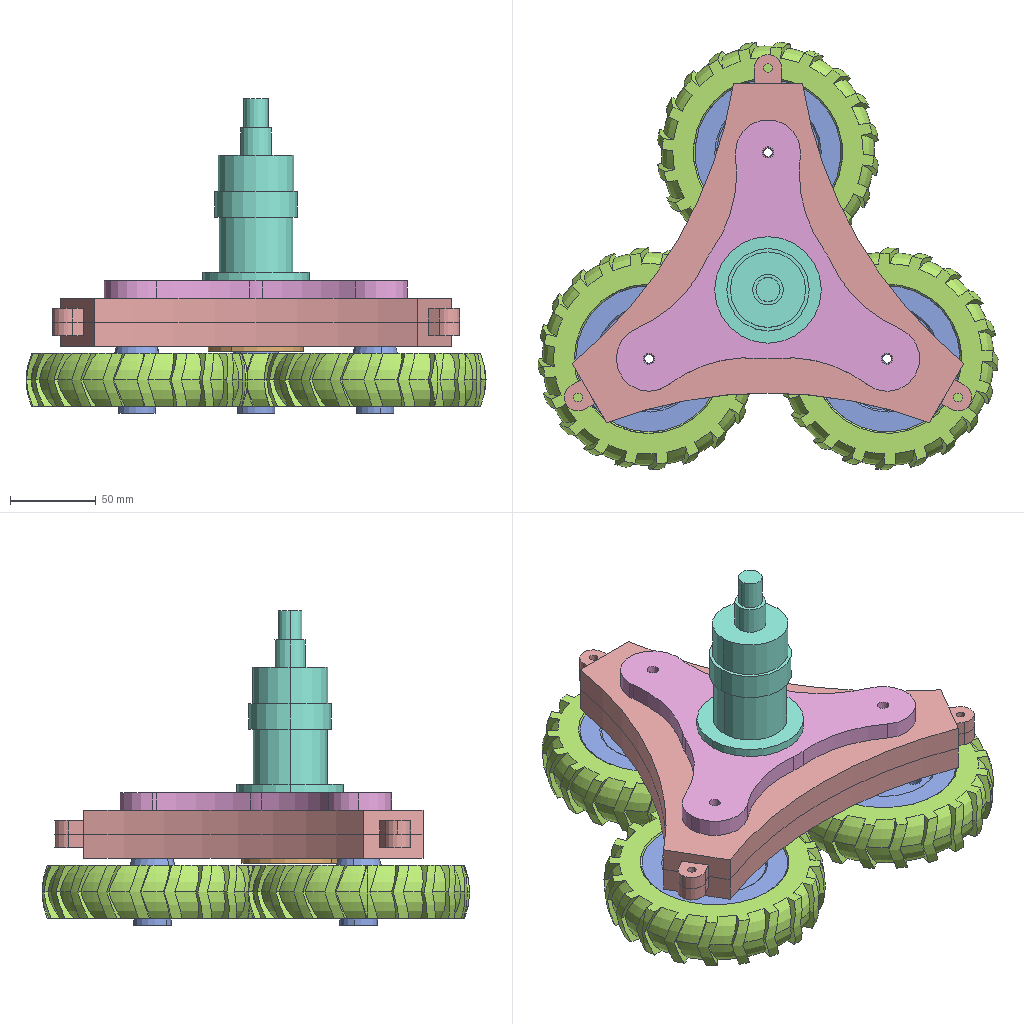Assembly | SolidWorks | 5 different items | 10 placed | box 268 x 249 x 183 mm
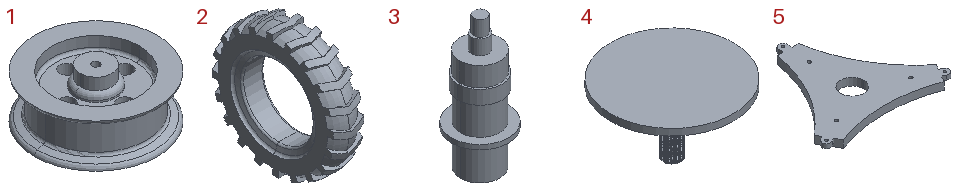Parts list (item | quantity | size | volume | features):
1 | x3 | 85 x 85 x 39 mm | 97267 mm3 | features ICE 6, Fillet 2, Blend 1, Chamfer 1, Extrusion 1, HoleWzd 1, RevCut 1
2 | x3 | 30.833 x 129 x 129 mm | 226597 mm3 | features CirPattern 1, ICE 1, RefAxis 1, RevCut 1, Revolution 1
3 | x1 | 62 x 62 x 144 mm | 181126 mm3 | features ICE 6, 3DProfileFeature 1, Cut 1, Extrusion 1, HoleWzd 1
4 | x1 | 56 x 56 x 31 mm | 8748 mm3 | features Extrusion 1, ICE 1, SweepThread 1
5 | x2 | 237.049 x 214.321 x 14 mm | 297445 mm3 | features ICE 3, 3DProfileFeature 2, HoleWzd 2, CirPattern 1, Extrusion 1
Mates (type | each side: item.copy, entity, surface, feature):
Coincident | 5.1 plane | assembly plane | 3 times
Concentric | 1.1 face cylinder Cut-Revolve3 | 2.1 face cylinder Revolve3
Coincident | 1.1 face plane Boss-Extrude1 | 2.1 face plane Revolve3
Concentric | 5.1 face cylinder Cut-Extrude2 | 1.1 face cylinder M6 Tapped Hole1
Coincident | 5.1 face plane Boss-Extrude1 | 5.2 face plane Boss-Extrude1
Concentric | 5.1 face cylinder Boss-Extrude2 | 5.2 face cylinder Boss-Extrude2
Concentric | 5.1 face cylinder CirPattern1 | 5.2 face cylinder CirPattern1
Coincident | 5.1 face plane Boss-Extrude1 | 1.1 face plane Loft2
Concentric | 3.1 face cylinder M8 Tapped Hole1 | 4.1 face cylinder Boss-Extrude2
Coincident | 3.1 face plane Boss-Extrude6 | 4.1 face plane Boss-Extrude1
Concentric | 5.1 face cylinder M6 Tapped Hole2 | assembly face
Coincident | 5.1 face plane CirPattern1 | assembly face
Concentric | assembly face | assembly face | 3 times
Concentric | 5.1 face cylinder Boss-Extrude2 | assembly face
Coincident | 5.1 face plane Boss-Extrude2 | assembly face
Coincident | 5.2 face plane Boss-Extrude2 | assembly face
Coincident | 1.1 face plane Boss-Extrude4 | assembly face
Coincident | assembly face | assembly face